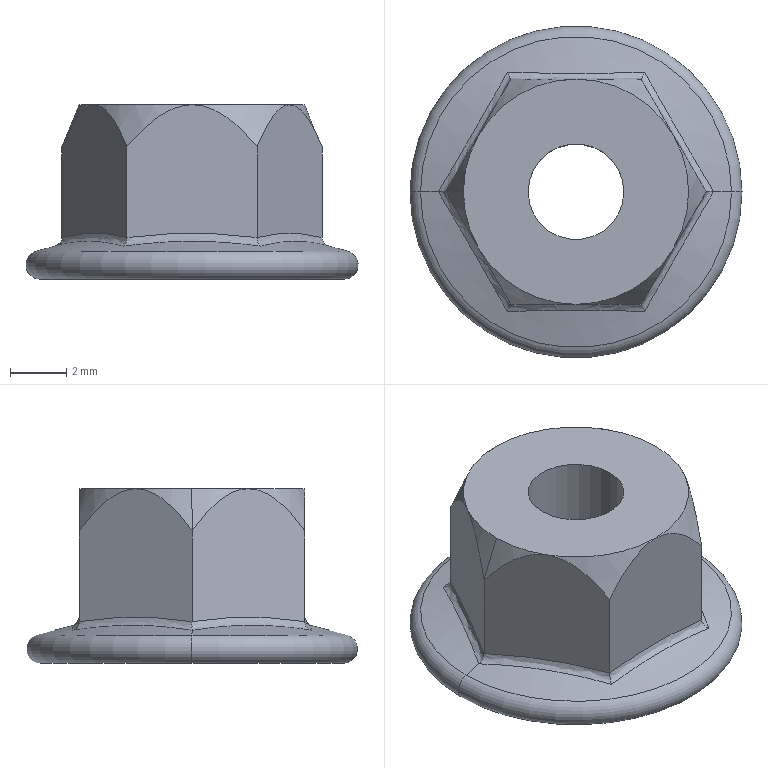Part | SolidWorks | features BaseBody 1 | 1 solid | 29 faces | box 11.8 x 11.8 x 6.2 mm | volume 341.044 mm3 | cone 11 | plane 8 | spline 6 | torus 2 | cylinder 2 | commonest cylinder face diameters 3.4 x2
STEP:
#1=CARTESIAN_POINT('',(2.444,4.233,-5.03));
#2=VERTEX_POINT('',#1);
#3=CARTESIAN_POINT('',(4.888,0.,-5.03));
#4=VERTEX_POINT('',#3);
#5=CARTESIAN_POINT('',(2.444,4.233,-5.03));
#6=CARTESIAN_POINT('',(2.548,4.05,-5.001));
#7=CARTESIAN_POINT('',(2.649,3.872,-4.976));
#8=CARTESIAN_POINT('',(2.799,3.608,-4.943));
#9=CARTESIAN_POINT('',(2.849,3.521,-4.933));
#10=CARTESIAN_POINT('',(2.923,3.39,-4.92));
#11=CARTESIAN_POINT('',(2.96,3.325,-4.913));
#12=CARTESIAN_POINT('',(2.997,3.261,-4.907));
#13=CARTESIAN_POINT('',(3.022,3.217,-4.903));
#14=CARTESIAN_POINT('',(3.034,3.197,-4.901));
#15=CARTESIAN_POINT('',(3.254,2.812,-4.867));
#16=CARTESIAN_POINT('',(3.451,2.468,-4.852));
#17=CARTESIAN_POINT('',(3.758,1.935,-4.851));
#18=CARTESIAN_POINT('',(3.859,1.76,-4.855));
#19=CARTESIAN_POINT('',(4.012,1.497,-4.867));
#20=CARTESIAN_POINT('',(4.063,1.409,-4.872));
#21=CARTESIAN_POINT('',(4.141,1.276,-4.881));
#22=CARTESIAN_POINT('',(4.18,1.21,-4.886));
#23=CARTESIAN_POINT('',(4.219,1.143,-4.891));
#24=CARTESIAN_POINT('',(4.245,1.098,-4.895));
#25=CARTESIAN_POINT('',(4.259,1.074,-4.897));
#26=CARTESIAN_POINT('',(4.472,0.709,-4.929));
#27=CARTESIAN_POINT('',(4.675,0.3632,-4.973));
#28=CARTESIAN_POINT('',(4.888,0.,-5.03));
#29=B_SPLINE_CURVE_WITH_KNOTS('',3,(#5,#6,#7,#8,#9,#10,#11,#12,#13,#14,#15,#16,#17,#18,#19,#20,#21,#22,#23,#24,#25,#26,#27,#28),.UNSPECIFIED.,.F.,.F.,(4,2,2,1,2,2,2,2,2,1,2,2,4),(0.,0.125,0.1875,0.2187,0.2344,0.25,0.5,0.625,0.6875,0.7187,0.7344,0.75,1.),.UNSPECIFIED.);
#30=EDGE_CURVE('',#2,#4,#29,.T.);
#31=ORIENTED_EDGE('',*,*,#30,.T.);
#32=CARTESIAN_POINT('',(5.523,0.,-5.2));
#33=VERTEX_POINT('',#32);
#34=CARTESIAN_POINT('',(4.619,0.,-4.958));
#35=DIRECTION('',(0.9659,0.,-0.2588));
#36=VECTOR('',#35,1000.);
#37=LINE('',#34,#36);
#38=EDGE_CURVE('',#4,#33,#37,.T.);
#39=ORIENTED_EDGE('',*,*,#38,.T.);
#40=CARTESIAN_POINT('',(-5.523,0.,-5.2));
#41=VERTEX_POINT('',#40);
#42=CARTESIAN_POINT('',(0.,0.,-5.2));
#43=DIRECTION('',(0.,0.,-1.));
#44=DIRECTION('',(-1.,0.,0.));
#45=AXIS2_PLACEMENT_3D('',#42,#43,#44);
#46=CIRCLE('',#45,5.523);
#47=EDGE_CURVE('',#41,#33,#46,.T.);
#48=ORIENTED_EDGE('',*,*,#47,.F.);
#49=CARTESIAN_POINT('',(-4.888,0.,-5.03));
#50=VERTEX_POINT('',#49);
#51=CARTESIAN_POINT('',(-4.619,0.,-4.958));
#52=DIRECTION('',(-0.9659,0.,-0.2588));
#53=VECTOR('',#52,1000.);
#54=LINE('',#51,#53);
#55=EDGE_CURVE('',#50,#41,#54,.T.);
#56=ORIENTED_EDGE('',*,*,#55,.F.);
#57=CARTESIAN_POINT('',(-2.444,4.233,-5.03));
#58=VERTEX_POINT('',#57);
#59=CARTESIAN_POINT('',(-4.888,0.,-5.03));
#60=CARTESIAN_POINT('',(-4.781,0.1813,-5.001));
#61=CARTESIAN_POINT('',(-4.677,0.3583,-4.976));
#62=CARTESIAN_POINT('',(-4.524,0.6202,-4.943));
#63=CARTESIAN_POINT('',(-4.473,0.7069,-4.933));
#64=CARTESIAN_POINT('',(-4.398,0.8363,-4.92));
#65=CARTESIAN_POINT('',(-4.36,0.9009,-4.913));
#66=CARTESIAN_POINT('',(-4.322,0.9654,-4.907));
#67=CARTESIAN_POINT('',(-4.297,1.008,-4.903));
#68=CARTESIAN_POINT('',(-4.285,1.029,-4.901));
#69=CARTESIAN_POINT('',(-4.062,1.412,-4.867));
#70=CARTESIAN_POINT('',(-3.862,1.755,-4.852));
#71=CARTESIAN_POINT('',(-3.555,2.287,-4.851));
#72=CARTESIAN_POINT('',(-3.454,2.462,-4.855));
#73=CARTESIAN_POINT('',(-3.303,2.726,-4.867));
#74=CARTESIAN_POINT('',(-3.252,2.814,-4.872));
#75=CARTESIAN_POINT('',(-3.176,2.948,-4.881));
#76=CARTESIAN_POINT('',(-3.138,3.015,-4.886));
#77=CARTESIAN_POINT('',(-3.099,3.082,-4.891));
#78=CARTESIAN_POINT('',(-3.073,3.127,-4.895));
#79=CARTESIAN_POINT('',(-3.06,3.151,-4.897));
#80=CARTESIAN_POINT('',(-2.85,3.518,-4.929));
#81=CARTESIAN_POINT('',(-2.652,3.867,-4.973));
#82=CARTESIAN_POINT('',(-2.444,4.233,-5.03));
#83=B_SPLINE_CURVE_WITH_KNOTS('',3,(#59,#60,#61,#62,#63,#64,#65,#66,#67,#68,#69,#70,#71,#72,#73,#74,#75,#76,#77,#78,#79,#80,#81,#82),.UNSPECIFIED.,.F.,.F.,(4,2,2,1,2,2,2,2,2,1,2,2,4),(0.,0.125,0.1875,0.2187,0.2344,0.25,0.5,0.625,0.6875,0.7187,0.7344,0.75,1.),.UNSPECIFIED.);
#84=EDGE_CURVE('',#50,#58,#83,.T.);
#85=ORIENTED_EDGE('',*,*,#84,.T.);
#86=CARTESIAN_POINT('',(-2.444,4.233,-5.03));
#87=CARTESIAN_POINT('',(-2.234,4.231,-5.001));
#88=CARTESIAN_POINT('',(-2.028,4.23,-4.976));
#89=CARTESIAN_POINT('',(-1.725,4.228,-4.943));
#90=CARTESIAN_POINT('',(-1.625,4.228,-4.933));
#91=CARTESIAN_POINT('',(-1.475,4.227,-4.92));
#92=CARTESIAN_POINT('',(-1.4,4.226,-4.913));
#93=CARTESIAN_POINT('',(-1.325,4.226,-4.907));
#94=CARTESIAN_POINT('',(-1.275,4.226,-4.903));
#95=CARTESIAN_POINT('',(-1.252,4.226,-4.901));
#96=CARTESIAN_POINT('',(-0.8085,4.224,-4.867));
#97=CARTESIAN_POINT('',(-0.4116,4.222,-4.852));
#98=CARTESIAN_POINT('',(0.2033,4.222,-4.851));
#99=CARTESIAN_POINT('',(0.4052,4.222,-4.855));
#100=CARTESIAN_POINT('',(0.7095,4.223,-4.867));
#101=CARTESIAN_POINT('',(0.8112,4.224,-4.872));
#102=CARTESIAN_POINT('',(0.965,4.224,-4.881));
#103=CARTESIAN_POINT('',(1.042,4.225,-4.886));
#104=CARTESIAN_POINT('',(1.12,4.225,-4.891));
#105=CARTESIAN_POINT('',(1.172,4.225,-4.895));
#106=CARTESIAN_POINT('',(1.199,4.225,-4.897));
#107=CARTESIAN_POINT('',(1.622,4.227,-4.929));
#108=CARTESIAN_POINT('',(2.023,4.23,-4.973));
#109=CARTESIAN_POINT('',(2.444,4.233,-5.03));
#110=B_SPLINE_CURVE_WITH_KNOTS('',3,(#86,#87,#88,#89,#90,#91,#92,#93,#94,#95,#96,#97,#98,#99,#100,#101,#102,#103,#104,#105,#106,#107,#108,#109),.UNSPECIFIED.,.F.,.F.,(4,2,2,1,2,2,2,2,2,1,2,2,4),(0.,0.125,0.1875,0.2188,0.2344,0.25,0.5,0.625,0.6875,0.7188,0.7344,0.75,1.),.UNSPECIFIED.);
#111=EDGE_CURVE('',#58,#2,#110,.T.);
#112=ORIENTED_EDGE('',*,*,#111,.T.);
#113=EDGE_LOOP('',(#31,#39,#48,#56,#85,#112));
#114=FACE_OUTER_BOUND('',#113,.T.);
#115=CARTESIAN_POINT('',(0.,0.,-4.958));
#116=DIRECTION('',(0.,0.,-1.));
#117=DIRECTION('',(-1.,0.,0.));
#118=AXIS2_PLACEMENT_3D('',#115,#116,#117);
#119=CONICAL_SURFACE('',#118,4.619,1.309);
#120=ADVANCED_FACE('',(#114),#119,.T.);
#121=ORIENTED_EDGE('',*,*,#47,.T.);
#122=CARTESIAN_POINT('',(5.391,0.,-6.2));
#123=VERTEX_POINT('',#122);
#124=CARTESIAN_POINT('',(5.391,0.,-5.691));
#125=DIRECTION('',(0.,1.,0.));
#126=DIRECTION('',(-1.,0.,0.));
#127=AXIS2_PLACEMENT_3D('',#124,#125,#126);
#128=CIRCLE('',#127,0.5087);
#129=EDGE_CURVE('',#33,#123,#128,.T.);
#130=ORIENTED_EDGE('',*,*,#129,.T.);
#131=CARTESIAN_POINT('',(-5.391,0.,-6.2));
#132=VERTEX_POINT('',#131);
#133=CARTESIAN_POINT('',(0.,0.,-6.2));
#134=DIRECTION('',(0.,0.,-1.));
#135=DIRECTION('',(-1.,0.,0.));
#136=AXIS2_PLACEMENT_3D('',#133,#134,#135);
#137=CIRCLE('',#136,5.391);
#138=EDGE_CURVE('',#132,#123,#137,.T.);
#139=ORIENTED_EDGE('',*,*,#138,.F.);
#140=CARTESIAN_POINT('',(-5.391,0.,-5.691));
#141=DIRECTION('',(0.,-1.,0.));
#142=DIRECTION('',(0.,0.,-1.));
#143=AXIS2_PLACEMENT_3D('',#140,#141,#142);
#144=CIRCLE('',#143,0.5087);
#145=EDGE_CURVE('',#41,#132,#144,.T.);
#146=ORIENTED_EDGE('',*,*,#145,.F.);
#147=EDGE_LOOP('',(#121,#130,#139,#146));
#148=FACE_OUTER_BOUND('',#147,.T.);
#149=CARTESIAN_POINT('',(0.,0.,-5.691));
#150=DIRECTION('',(0.,0.,-1.));
#151=DIRECTION('',(-1.,0.,0.));
#152=AXIS2_PLACEMENT_3D('',#149,#150,#151);
#153=TOROIDAL_SURFACE('',#152,5.391,0.5087);
#154=ADVANCED_FACE('',(#148),#153,.T.);
#155=CARTESIAN_POINT('',(1.7,0.,-5.714));
#156=VERTEX_POINT('',#155);
#157=CARTESIAN_POINT('',(-1.7,0.,-5.714));
#158=VERTEX_POINT('',#157);
#159=CARTESIAN_POINT('',(0.,0.,-5.714));
#160=DIRECTION('',(0.,0.,-1.));
#161=DIRECTION('',(1.,0.,0.));
#162=AXIS2_PLACEMENT_3D('',#159,#160,#161);
#163=CIRCLE('',#162,1.7);
#164=EDGE_CURVE('',#156,#158,#163,.T.);
#165=ORIENTED_EDGE('',*,*,#164,.F.);
#166=CARTESIAN_POINT('',(2.186,0.,-6.2));
#167=VERTEX_POINT('',#166);
#168=CARTESIAN_POINT('',(2.186,0.,-6.2));
#169=DIRECTION('',(0.7071,0.,-0.7071));
#170=VECTOR('',#169,1000.);
#171=LINE('',#168,#170);
#172=EDGE_CURVE('',#156,#167,#171,.T.);
#173=ORIENTED_EDGE('',*,*,#172,.T.);
#174=CARTESIAN_POINT('',(-2.186,0.,-6.2));
#175=VERTEX_POINT('',#174);
#176=CARTESIAN_POINT('',(0.,0.,-6.2));
#177=DIRECTION('',(0.,0.,1.));
#178=DIRECTION('',(1.,0.,0.));
#179=AXIS2_PLACEMENT_3D('',#176,#177,#178);
#180=CIRCLE('',#179,2.186);
#181=EDGE_CURVE('',#175,#167,#180,.T.);
#182=ORIENTED_EDGE('',*,*,#181,.F.);
#183=CARTESIAN_POINT('',(-2.186,0.,-6.2));
#184=DIRECTION('',(-0.7071,0.,-0.7071));
#185=VECTOR('',#184,1000.);
#186=LINE('',#183,#185);
#187=EDGE_CURVE('',#158,#175,#186,.T.);
#188=ORIENTED_EDGE('',*,*,#187,.F.);
#189=EDGE_LOOP('',(#165,#173,#182,#188));
#190=FACE_OUTER_BOUND('',#189,.T.);
#191=CARTESIAN_POINT('',(0.,0.,-6.2));
#192=DIRECTION('',(0.,0.,-1.));
#193=DIRECTION('',(-1.,0.,0.));
#194=AXIS2_PLACEMENT_3D('',#191,#192,#193);
#195=CONICAL_SURFACE('',#194,2.186,0.7854);
#196=ADVANCED_FACE('',(#190),#195,.F.);
#197=ORIENTED_EDGE('',*,*,#164,.T.);
#198=CARTESIAN_POINT('',(-1.7,0.,0.));
#199=VERTEX_POINT('',#198);
#200=CARTESIAN_POINT('',(-1.7,0.,-6.2));
#201=DIRECTION('',(0.,0.,1.));
#202=VECTOR('',#201,1000.);
#203=LINE('',#200,#202);
#204=EDGE_CURVE('',#158,#199,#203,.T.);
#205=ORIENTED_EDGE('',*,*,#204,.T.);
#206=CARTESIAN_POINT('',(1.7,0.,0.));
#207=VERTEX_POINT('',#206);
#208=CARTESIAN_POINT('',(0.,0.,0.));
#209=DIRECTION('',(0.,0.,1.));
#210=DIRECTION('',(1.,0.,0.));
#211=AXIS2_PLACEMENT_3D('',#208,#209,#210);
#212=CIRCLE('',#211,1.7);
#213=EDGE_CURVE('',#199,#207,#212,.T.);
#214=ORIENTED_EDGE('',*,*,#213,.T.);
#215=CARTESIAN_POINT('',(1.7,0.,-6.2));
#216=DIRECTION('',(0.,0.,1.));
#217=VECTOR('',#216,1000.);
#218=LINE('',#215,#217);
#219=EDGE_CURVE('',#156,#207,#218,.T.);
#220=ORIENTED_EDGE('',*,*,#219,.F.);
#221=EDGE_LOOP('',(#197,#205,#214,#220));
#222=FACE_OUTER_BOUND('',#221,.T.);
#223=CARTESIAN_POINT('',(0.,0.,-6.2));
#224=DIRECTION('',(0.,0.,1.));
#225=DIRECTION('',(1.,0.,0.));
#226=AXIS2_PLACEMENT_3D('',#223,#224,#225);
#227=CYLINDRICAL_SURFACE('',#226,1.7);
#228=ADVANCED_FACE('',(#222),#227,.F.);
#229=CARTESIAN_POINT('',(-3.464,-2.,0.));
#230=VERTEX_POINT('',#229);
#231=CARTESIAN_POINT('',(-4.,0.,0.));
#232=VERTEX_POINT('',#231);
#233=CARTESIAN_POINT('',(0.,0.,0.));
#234=DIRECTION('',(0.,0.,-1.));
#235=DIRECTION('',(1.,0.,0.));
#236=AXIS2_PLACEMENT_3D('',#233,#234,#235);
#237=CIRCLE('',#236,4.);
#238=EDGE_CURVE('',#230,#232,#237,.T.);
#239=ORIENTED_EDGE('',*,*,#238,.T.);
#240=CARTESIAN_POINT('',(-4.619,0.,-1.5));
#241=VERTEX_POINT('',#240);
#242=CARTESIAN_POINT('',(-4.,0.,0.));
#243=DIRECTION('',(-0.3814,0.,-0.9244));
#244=VECTOR('',#243,1000.);
#245=LINE('',#242,#244);
#246=EDGE_CURVE('',#232,#241,#245,.T.);
#247=ORIENTED_EDGE('',*,*,#246,.T.);
#248=CARTESIAN_POINT('',(-4.619,0.,-1.5));
#249=CARTESIAN_POINT('',(-4.543,-0.1306,-1.317));
#250=CARTESIAN_POINT('',(-4.465,-0.2661,-1.141));
#251=CARTESIAN_POINT('',(-4.3,-0.5524,-0.8063));
#252=CARTESIAN_POINT('',(-4.213,-0.703,-0.6482));
#253=CARTESIAN_POINT('',(-4.024,-1.03,-0.3637));
#254=CARTESIAN_POINT('',(-3.922,-1.208,-0.2367));
#255=CARTESIAN_POINT('',(-3.703,-1.587,-0.05468));
#256=CARTESIAN_POINT('',(-3.584,-1.792,0.));
#257=CARTESIAN_POINT('',(-3.464,-2.,0.));
#258=B_SPLINE_CURVE_WITH_KNOTS('',3,(#248,#249,#250,#251,#252,#253,#254,#255,#256,#257),.UNSPECIFIED.,.F.,.F.,(4,2,2,2,4),(0.,0.0007048,0.00141,0.002115,0.002819),.UNSPECIFIED.);
#259=EDGE_CURVE('',#241,#230,#258,.T.);
#260=ORIENTED_EDGE('',*,*,#259,.T.);
#261=EDGE_LOOP('',(#239,#247,#260));
#262=FACE_OUTER_BOUND('',#261,.T.);
#263=CARTESIAN_POINT('',(0.,0.,0.));
#264=DIRECTION('',(0.,0.,-1.));
#265=DIRECTION('',(-1.,0.,0.));
#266=AXIS2_PLACEMENT_3D('',#263,#264,#265);
#267=CONICAL_SURFACE('',#266,4.,0.3913);
#268=ADVANCED_FACE('',(#262),#267,.T.);
#269=CARTESIAN_POINT('',(-4.619,0.,-4.717));
#270=VERTEX_POINT('',#269);
#271=CARTESIAN_POINT('',(-4.888,0.,-5.03));
#272=CARTESIAN_POINT('',(-4.853,0.,-5.021));
#273=CARTESIAN_POINT('',(-4.818,-0.000409,-5.006));
#274=CARTESIAN_POINT('',(-4.77,0.0002124,-4.977));
#275=CARTESIAN_POINT('',(-4.755,0.000207,-4.967));
#276=CARTESIAN_POINT('',(-4.733,0.0001255,-4.949));
#277=CARTESIAN_POINT('',(-4.726,0.00008611,-4.943));
#278=CARTESIAN_POINT('',(-4.713,0.00002162,-4.931));
#279=CARTESIAN_POINT('',(-4.707,-0.000003411,-4.925));
#280=CARTESIAN_POINT('',(-4.644,-0.000002588,-4.855));
#281=CARTESIAN_POINT('',(-4.619,0.000006557,-4.78));
#282=CARTESIAN_POINT('',(-4.619,0.,-4.717));
#283=B_SPLINE_CURVE_WITH_KNOTS('',3,(#271,#272,#273,#274,#275,#276,#277,#278,#279,#280,#281,#282),.UNSPECIFIED.,.F.,.F.,(4,2,2,2,2,4),(0.,0.25,0.375,0.4375,0.5,1.),.UNSPECIFIED.);
#284=EDGE_CURVE('',#50,#270,#283,.T.);
#285=ORIENTED_EDGE('',*,*,#284,.T.);
#286=CARTESIAN_POINT('',(-2.309,4.,-4.717));
#287=VERTEX_POINT('',#286);
#288=CARTESIAN_POINT('',(-2.309,4.,-4.717));
#289=CARTESIAN_POINT('',(-2.693,3.336,-4.62));
#290=CARTESIAN_POINT('',(-3.077,2.67,-4.562));
#291=CARTESIAN_POINT('',(-3.851,1.33,-4.562));
#292=CARTESIAN_POINT('',(-4.235,0.664,-4.62));
#293=CARTESIAN_POINT('',(-4.619,0.,-4.717));
#294=B_SPLINE_CURVE_WITH_KNOTS('',3,(#288,#289,#290,#291,#292,#293),.UNSPECIFIED.,.F.,.F.,(4,2,4),(0.,0.002315,0.004629),.UNSPECIFIED.);
#295=EDGE_CURVE('',#287,#270,#294,.T.);
#296=ORIENTED_EDGE('',*,*,#295,.F.);
#297=CARTESIAN_POINT('',(-2.309,4.,-4.717));
#298=CARTESIAN_POINT('',(-2.309,4.,-4.749));
#299=CARTESIAN_POINT('',(-2.312,4.005,-4.783));
#300=CARTESIAN_POINT('',(-2.322,4.023,-4.835));
#301=CARTESIAN_POINT('',(-2.326,4.03,-4.852));
#302=CARTESIAN_POINT('',(-2.334,4.043,-4.877));
#303=CARTESIAN_POINT('',(-2.339,4.051,-4.89));
#304=CARTESIAN_POINT('',(-2.344,4.06,-4.904));
#305=CARTESIAN_POINT('',(-2.347,4.065,-4.91));
#306=CARTESIAN_POINT('',(-2.348,4.068,-4.914));
#307=CARTESIAN_POINT('',(-2.35,4.07,-4.917));
#308=CARTESIAN_POINT('',(-2.355,4.079,-4.929));
#309=CARTESIAN_POINT('',(-2.364,4.096,-4.948));
#310=CARTESIAN_POINT('',(-2.395,4.148,-4.991));
#311=CARTESIAN_POINT('',(-2.417,4.185,-5.015));
#312=CARTESIAN_POINT('',(-2.444,4.233,-5.03));
#313=B_SPLINE_CURVE_WITH_KNOTS('',3,(#297,#298,#299,#300,#301,#302,#303,#304,#305,#306,#307,#308,#309,#310,#311,#312),.UNSPECIFIED.,.F.,.F.,(4,2,2,1,1,2,2,2,4),(0.,0.25,0.375,0.4375,0.4688,0.4844,0.5,0.75,1.),.UNSPECIFIED.);
#314=EDGE_CURVE('',#287,#58,#313,.T.);
#315=ORIENTED_EDGE('',*,*,#314,.T.);
#316=ORIENTED_EDGE('',*,*,#84,.F.);
#317=EDGE_LOOP('',(#285,#296,#315,#316));
#318=FACE_OUTER_BOUND('',#317,.T.);
#319=CARTESIAN_POINT('',(-2.208,4.175,-4.744));
#320=CARTESIAN_POINT('',(-2.224,4.148,-4.981));
#321=CARTESIAN_POINT('',(-2.429,4.258,-5.034));
#322=CARTESIAN_POINT('',(-2.62,3.463,-4.633));
#323=CARTESIAN_POINT('',(-2.628,3.447,-4.867));
#324=CARTESIAN_POINT('',(-2.831,3.551,-4.922));
#325=CARTESIAN_POINT('',(-3.036,2.742,-4.562));
#326=CARTESIAN_POINT('',(-3.042,2.732,-4.792));
#327=CARTESIAN_POINT('',(-3.236,2.84,-4.852));
#328=CARTESIAN_POINT('',(-3.883,1.275,-4.561));
#329=CARTESIAN_POINT('',(-3.877,1.285,-4.791));
#330=CARTESIAN_POINT('',(-4.068,1.399,-4.851));
#331=CARTESIAN_POINT('',(-4.303,0.5472,-4.631));
#332=CARTESIAN_POINT('',(-4.294,0.5622,-4.865));
#333=CARTESIAN_POINT('',(-4.485,0.6866,-4.921));
#334=CARTESIAN_POINT('',(-4.72,-0.1757,-4.744));
#335=CARTESIAN_POINT('',(-4.704,-0.148,-4.981));
#336=CARTESIAN_POINT('',(-4.902,-0.02532,-5.034));
#337=(BOUNDED_SURFACE()B_SPLINE_SURFACE(3,2,((#319,#320,#321),(#322,#323,#324),(#325,#326,#327),(#328,#329,#330),(#331,#332,#333),(#334,#335,#336)),.UNSPECIFIED.,.F.,.F.,.T.)B_SPLINE_SURFACE_WITH_KNOTS((4,2,4),(3,3),(0.0205,0.02298,0.02547),(0.,1.),.UNSPECIFIED.)GEOMETRIC_REPRESENTATION_ITEM()RATIONAL_B_SPLINE_SURFACE(((1.,0.7821,1.),(1.,0.7882,1.),(1.,0.7933,1.),(1.,0.7934,1.),(1.,0.7883,1.),(1.,0.7821,1.)))REPRESENTATION_ITEM('')SURFACE());
#338=ADVANCED_FACE('',(#318),#337,.F.);
#339=CARTESIAN_POINT('',(2.309,4.,-4.717));
#340=VERTEX_POINT('',#339);
#341=CARTESIAN_POINT('',(2.309,4.,-4.717));
#342=CARTESIAN_POINT('',(2.309,4.,-4.749));
#343=CARTESIAN_POINT('',(2.313,4.005,-4.783));
#344=CARTESIAN_POINT('',(2.323,4.022,-4.835));
#345=CARTESIAN_POINT('',(2.327,4.03,-4.852));
#346=CARTESIAN_POINT('',(2.335,4.043,-4.877));
#347=CARTESIAN_POINT('',(2.339,4.051,-4.89));
#348=CARTESIAN_POINT('',(2.344,4.06,-4.904));
#349=CARTESIAN_POINT('',(2.347,4.065,-4.91));
#350=CARTESIAN_POINT('',(2.348,4.068,-4.914));
#351=CARTESIAN_POINT('',(2.35,4.07,-4.917));
#352=CARTESIAN_POINT('',(2.355,4.079,-4.929));
#353=CARTESIAN_POINT('',(2.365,4.095,-4.948));
#354=CARTESIAN_POINT('',(2.395,4.148,-4.991));
#355=CARTESIAN_POINT('',(2.416,4.186,-5.015));
#356=CARTESIAN_POINT('',(2.444,4.233,-5.03));
#357=B_SPLINE_CURVE_WITH_KNOTS('',3,(#341,#342,#343,#344,#345,#346,#347,#348,#349,#350,#351,#352,#353,#354,#355,#356),.UNSPECIFIED.,.F.,.F.,(4,2,2,1,1,2,2,2,4),(0.,0.25,0.375,0.4375,0.4687,0.4844,0.5,0.75,1.),.UNSPECIFIED.);
#358=EDGE_CURVE('',#340,#2,#357,.T.);
#359=ORIENTED_EDGE('',*,*,#358,.T.);
#360=ORIENTED_EDGE('',*,*,#111,.F.);
#361=ORIENTED_EDGE('',*,*,#314,.F.);
#362=CARTESIAN_POINT('',(2.309,4.,-4.717));
#363=CARTESIAN_POINT('',(1.543,4.,-4.62));
#364=CARTESIAN_POINT('',(0.7733,4.,-4.562));
#365=CARTESIAN_POINT('',(-0.7733,4.,-4.562));
#366=CARTESIAN_POINT('',(-1.543,4.,-4.62));
#367=CARTESIAN_POINT('',(-2.309,4.,-4.717));
#368=B_SPLINE_CURVE_WITH_KNOTS('',3,(#362,#363,#364,#365,#366,#367),.UNSPECIFIED.,.F.,.F.,(4,2,4),(0.,0.002315,0.004629),.UNSPECIFIED.);
#369=EDGE_CURVE('',#340,#287,#368,.T.);
#370=ORIENTED_EDGE('',*,*,#369,.F.);
#371=EDGE_LOOP('',(#359,#360,#361,#370));
#372=FACE_OUTER_BOUND('',#371,.T.);
#373=CARTESIAN_POINT('',(2.512,4.,-4.744));
#374=CARTESIAN_POINT('',(2.48,4.,-4.981));
#375=CARTESIAN_POINT('',(2.473,4.233,-5.034));
#376=CARTESIAN_POINT('',(1.689,4.,-4.633));
#377=CARTESIAN_POINT('',(1.671,4.,-4.867));
#378=CARTESIAN_POINT('',(1.659,4.227,-4.922));
#379=CARTESIAN_POINT('',(0.8571,4.,-4.562));
#380=CARTESIAN_POINT('',(0.8448,4.,-4.792));
#381=CARTESIAN_POINT('',(0.8416,4.222,-4.852));
#382=CARTESIAN_POINT('',(-0.8378,4.,-4.561));
#383=CARTESIAN_POINT('',(-0.8257,4.,-4.791));
#384=CARTESIAN_POINT('',(-0.8227,4.222,-4.851));
#385=CARTESIAN_POINT('',(-1.678,4.,-4.631));
#386=CARTESIAN_POINT('',(-1.66,4.,-4.865));
#387=CARTESIAN_POINT('',(-1.648,4.227,-4.921));
#388=CARTESIAN_POINT('',(-2.512,4.,-4.744));
#389=CARTESIAN_POINT('',(-2.48,4.,-4.981));
#390=CARTESIAN_POINT('',(-2.473,4.233,-5.034));
#391=(BOUNDED_SURFACE()B_SPLINE_SURFACE(3,2,((#373,#374,#375),(#376,#377,#378),(#379,#380,#381),(#382,#383,#384),(#385,#386,#387),(#388,#389,#390)),.UNSPECIFIED.,.F.,.F.,.T.)B_SPLINE_SURFACE_WITH_KNOTS((4,2,4),(3,3),(0.02046,0.02295,0.02543),(0.,1.),.UNSPECIFIED.)GEOMETRIC_REPRESENTATION_ITEM()RATIONAL_B_SPLINE_SURFACE(((1.,0.7821,1.),(1.,0.7882,1.),(1.,0.7933,1.),(1.,0.7934,1.),(1.,0.7883,1.),(1.,0.7821,1.)))REPRESENTATION_ITEM('')SURFACE());
#392=ADVANCED_FACE('',(#372),#391,.F.);
#393=CARTESIAN_POINT('',(-2.444,-4.233,-5.03));
#394=VERTEX_POINT('',#393);
#395=CARTESIAN_POINT('',(-2.309,-4.,-4.717));
#396=VERTEX_POINT('',#395);
#397=CARTESIAN_POINT('',(-2.444,-4.233,-5.03));
#398=CARTESIAN_POINT('',(-2.427,-4.203,-5.021));
#399=CARTESIAN_POINT('',(-2.408,-4.172,-5.006));
#400=CARTESIAN_POINT('',(-2.385,-4.131,-4.977));
#401=CARTESIAN_POINT('',(-2.377,-4.117,-4.967));
#402=CARTESIAN_POINT('',(-2.367,-4.099,-4.949));
#403=CARTESIAN_POINT('',(-2.363,-4.093,-4.943));
#404=CARTESIAN_POINT('',(-2.356,-4.081,-4.931));
#405=CARTESIAN_POINT('',(-2.354,-4.077,-4.925));
#406=CARTESIAN_POINT('',(-2.322,-4.022,-4.855));
#407=CARTESIAN_POINT('',(-2.309,-4.,-4.78));
#408=CARTESIAN_POINT('',(-2.309,-4.,-4.717));
#409=B_SPLINE_CURVE_WITH_KNOTS('',3,(#397,#398,#399,#400,#401,#402,#403,#404,#405,#406,#407,#408),.UNSPECIFIED.,.F.,.F.,(4,2,2,2,2,4),(0.,0.25,0.375,0.4375,0.5,1.),.UNSPECIFIED.);
#410=EDGE_CURVE('',#394,#396,#409,.T.);
#411=ORIENTED_EDGE('',*,*,#410,.T.);
#412=CARTESIAN_POINT('',(-4.619,0.,-4.717));
#413=CARTESIAN_POINT('',(-4.235,-0.664,-4.62));
#414=CARTESIAN_POINT('',(-3.851,-1.33,-4.562));
#415=CARTESIAN_POINT('',(-3.077,-2.67,-4.562));
#416=CARTESIAN_POINT('',(-2.693,-3.336,-4.62));
#417=CARTESIAN_POINT('',(-2.309,-4.,-4.717));
#418=B_SPLINE_CURVE_WITH_KNOTS('',3,(#412,#413,#414,#415,#416,#417),.UNSPECIFIED.,.F.,.F.,(4,2,4),(0.,0.002315,0.004629),.UNSPECIFIED.);
#419=EDGE_CURVE('',#270,#396,#418,.T.);
#420=ORIENTED_EDGE('',*,*,#419,.F.);
#421=ORIENTED_EDGE('',*,*,#284,.F.);
#422=CARTESIAN_POINT('',(-2.444,-4.233,-5.03));
#423=CARTESIAN_POINT('',(-2.548,-4.05,-5.001));
#424=CARTESIAN_POINT('',(-2.649,-3.872,-4.976));
#425=CARTESIAN_POINT('',(-2.799,-3.608,-4.943));
#426=CARTESIAN_POINT('',(-2.849,-3.521,-4.933));
#427=CARTESIAN_POINT('',(-2.923,-3.39,-4.92));
#428=CARTESIAN_POINT('',(-2.96,-3.325,-4.913));
#429=CARTESIAN_POINT('',(-2.997,-3.261,-4.907));
#430=CARTESIAN_POINT('',(-3.022,-3.217,-4.903));
#431=CARTESIAN_POINT('',(-3.034,-3.197,-4.901));
#432=CARTESIAN_POINT('',(-3.254,-2.812,-4.867));
#433=CARTESIAN_POINT('',(-3.451,-2.468,-4.852));
#434=CARTESIAN_POINT('',(-3.758,-1.935,-4.851));
#435=CARTESIAN_POINT('',(-3.859,-1.76,-4.855));
#436=CARTESIAN_POINT('',(-4.012,-1.497,-4.867));
#437=CARTESIAN_POINT('',(-4.063,-1.409,-4.872));
#438=CARTESIAN_POINT('',(-4.141,-1.276,-4.881));
#439=CARTESIAN_POINT('',(-4.18,-1.21,-4.886));
#440=CARTESIAN_POINT('',(-4.219,-1.143,-4.891));
#441=CARTESIAN_POINT('',(-4.245,-1.098,-4.895));
#442=CARTESIAN_POINT('',(-4.259,-1.074,-4.897));
#443=CARTESIAN_POINT('',(-4.472,-0.709,-4.929));
#444=CARTESIAN_POINT('',(-4.675,-0.3632,-4.973));
#445=CARTESIAN_POINT('',(-4.888,0.,-5.03));
#446=B_SPLINE_CURVE_WITH_KNOTS('',3,(#422,#423,#424,#425,#426,#427,#428,#429,#430,#431,#432,#433,#434,#435,#436,#437,#438,#439,#440,#441,#442,#443,#444,#445),.UNSPECIFIED.,.F.,.F.,(4,2,2,1,2,2,2,2,2,1,2,2,4),(0.,0.125,0.1875,0.2188,0.2344,0.25,0.5,0.625,0.6875,0.7188,0.7344,0.75,1.),.UNSPECIFIED.);
#447=EDGE_CURVE('',#394,#50,#446,.T.);
#448=ORIENTED_EDGE('',*,*,#447,.F.);
#449=EDGE_LOOP('',(#411,#420,#421,#448));
#450=FACE_OUTER_BOUND('',#449,.T.);
#451=CARTESIAN_POINT('',(-4.72,0.1754,-4.744));
#452=CARTESIAN_POINT('',(-4.704,0.1476,-4.981));
#453=CARTESIAN_POINT('',(-4.902,0.02496,-5.034));
#454=CARTESIAN_POINT('',(-4.309,-0.5372,-4.633));
#455=CARTESIAN_POINT('',(-4.3,-0.5525,-4.867));
#456=CARTESIAN_POINT('',(-4.491,-0.6768,-4.922));
#457=CARTESIAN_POINT('',(-3.893,-1.258,-4.562));
#458=CARTESIAN_POINT('',(-3.887,-1.268,-4.792));
#459=CARTESIAN_POINT('',(-4.078,-1.382,-4.852));
#460=CARTESIAN_POINT('',(-3.045,-2.725,-4.561));
#461=CARTESIAN_POINT('',(-3.051,-2.715,-4.791));
#462=CARTESIAN_POINT('',(-3.245,-2.823,-4.851));
#463=CARTESIAN_POINT('',(-2.625,-3.453,-4.631));
#464=CARTESIAN_POINT('',(-2.634,-3.438,-4.865));
#465=CARTESIAN_POINT('',(-2.837,-3.541,-4.921));
#466=CARTESIAN_POINT('',(-2.208,-4.176,-4.744));
#467=CARTESIAN_POINT('',(-2.224,-4.148,-4.981));
#468=CARTESIAN_POINT('',(-2.429,-4.258,-5.034));
#469=(BOUNDED_SURFACE()B_SPLINE_SURFACE(3,2,((#451,#452,#453),(#454,#455,#456),(#457,#458,#459),(#460,#461,#462),(#463,#464,#465),(#466,#467,#468)),.UNSPECIFIED.,.F.,.F.,.T.)B_SPLINE_SURFACE_WITH_KNOTS((4,2,4),(3,3),(0.0205,0.02298,0.02547),(0.,1.),.UNSPECIFIED.)GEOMETRIC_REPRESENTATION_ITEM()RATIONAL_B_SPLINE_SURFACE(((1.,0.7821,1.),(1.,0.7882,1.),(1.,0.7933,1.),(1.,0.7934,1.),(1.,0.7883,1.),(1.,0.7821,1.)))REPRESENTATION_ITEM('')SURFACE());
#470=ADVANCED_FACE('',(#450),#469,.F.);
#471=CARTESIAN_POINT('',(4.619,0.,-4.717));
#472=VERTEX_POINT('',#471);
#473=CARTESIAN_POINT('',(4.619,0.,-4.717));
#474=CARTESIAN_POINT('',(4.619,0.000005018,-4.749));
#475=CARTESIAN_POINT('',(4.625,-0.000302,-4.783));
#476=CARTESIAN_POINT('',(4.645,-0.0003222,-4.835));
#477=CARTESIAN_POINT('',(4.653,-0.0002683,-4.852));
#478=CARTESIAN_POINT('',(4.669,-0.0001491,-4.877));
#479=CARTESIAN_POINT('',(4.677,-0.00008204,-4.89));
#480=CARTESIAN_POINT('',(4.688,-0.00002565,-4.904));
#481=CARTESIAN_POINT('',(4.694,-0.0000114,-4.91));
#482=CARTESIAN_POINT('',(4.697,-0.00000472,-4.914));
#483=CARTESIAN_POINT('',(4.7,-0.000002661,-4.917));
#484=CARTESIAN_POINT('',(4.71,-0.000001503,-4.929));
#485=CARTESIAN_POINT('',(4.729,-0.0005767,-4.948));
#486=CARTESIAN_POINT('',(4.79,-0.0004463,-4.991));
#487=CARTESIAN_POINT('',(4.833,0.0006583,-5.015));
#488=CARTESIAN_POINT('',(4.888,0.,-5.03));
#489=B_SPLINE_CURVE_WITH_KNOTS('',3,(#473,#474,#475,#476,#477,#478,#479,#480,#481,#482,#483,#484,#485,#486,#487,#488),.UNSPECIFIED.,.F.,.F.,(4,2,2,1,1,2,2,2,4),(0.,0.25,0.375,0.4375,0.4688,0.4844,0.5,0.75,1.),.UNSPECIFIED.);
#490=EDGE_CURVE('',#472,#4,#489,.T.);
#491=ORIENTED_EDGE('',*,*,#490,.T.);
#492=ORIENTED_EDGE('',*,*,#30,.F.);
#493=ORIENTED_EDGE('',*,*,#358,.F.);
#494=CARTESIAN_POINT('',(4.619,0.,-4.717));
#495=CARTESIAN_POINT('',(4.235,0.664,-4.62));
#496=CARTESIAN_POINT('',(3.851,1.33,-4.562));
#497=CARTESIAN_POINT('',(3.077,2.67,-4.562));
#498=CARTESIAN_POINT('',(2.693,3.336,-4.62));
#499=CARTESIAN_POINT('',(2.309,4.,-4.717));
#500=B_SPLINE_CURVE_WITH_KNOTS('',3,(#494,#495,#496,#497,#498,#499),.UNSPECIFIED.,.F.,.F.,(4,2,4),(0.,0.002315,0.004629),.UNSPECIFIED.);
#501=EDGE_CURVE('',#472,#340,#500,.T.);
#502=ORIENTED_EDGE('',*,*,#501,.F.);
#503=EDGE_LOOP('',(#491,#492,#493,#502));
#504=FACE_OUTER_BOUND('',#503,.T.);
#505=CARTESIAN_POINT('',(4.72,-0.1754,-4.744));
#506=CARTESIAN_POINT('',(4.704,-0.1476,-4.981));
#507=CARTESIAN_POINT('',(4.902,-0.02496,-5.034));
#508=CARTESIAN_POINT('',(4.309,0.5372,-4.633));
#509=CARTESIAN_POINT('',(4.3,0.5525,-4.867));
#510=CARTESIAN_POINT('',(4.491,0.6768,-4.922));
#511=CARTESIAN_POINT('',(3.893,1.258,-4.562));
#512=CARTESIAN_POINT('',(3.887,1.268,-4.792));
#513=CARTESIAN_POINT('',(4.078,1.382,-4.852));
#514=CARTESIAN_POINT('',(3.045,2.725,-4.561));
#515=CARTESIAN_POINT('',(3.051,2.715,-4.791));
#516=CARTESIAN_POINT('',(3.245,2.823,-4.851));
#517=CARTESIAN_POINT('',(2.625,3.453,-4.631));
#518=CARTESIAN_POINT('',(2.634,3.438,-4.865));
#519=CARTESIAN_POINT('',(2.837,3.541,-4.921));
#520=CARTESIAN_POINT('',(2.208,4.176,-4.744));
#521=CARTESIAN_POINT('',(2.224,4.148,-4.981));
#522=CARTESIAN_POINT('',(2.429,4.258,-5.034));
#523=(BOUNDED_SURFACE()B_SPLINE_SURFACE(3,2,((#505,#506,#507),(#508,#509,#510),(#511,#512,#513),(#514,#515,#516),(#517,#518,#519),(#520,#521,#522)),.UNSPECIFIED.,.F.,.F.,.T.)B_SPLINE_SURFACE_WITH_KNOTS((4,2,4),(3,3),(0.0205,0.02298,0.02547),(0.,1.),.UNSPECIFIED.)GEOMETRIC_REPRESENTATION_ITEM()RATIONAL_B_SPLINE_SURFACE(((1.,0.7821,1.),(1.,0.7882,1.),(1.,0.7933,1.),(1.,0.7934,1.),(1.,0.7883,1.),(1.,0.7821,1.)))REPRESENTATION_ITEM('')SURFACE());
#524=ADVANCED_FACE('',(#504),#523,.F.);
#525=CARTESIAN_POINT('',(2.444,-4.233,-5.03));
#526=VERTEX_POINT('',#525);
#527=CARTESIAN_POINT('',(2.309,-4.,-4.717));
#528=VERTEX_POINT('',#527);
#529=CARTESIAN_POINT('',(2.444,-4.233,-5.03));
#530=CARTESIAN_POINT('',(2.427,-4.203,-5.021));
#531=CARTESIAN_POINT('',(2.409,-4.172,-5.006));
#532=CARTESIAN_POINT('',(2.385,-4.131,-4.977));
#533=CARTESIAN_POINT('',(2.377,-4.118,-4.967));
#534=CARTESIAN_POINT('',(2.366,-4.099,-4.949));
#535=CARTESIAN_POINT('',(2.363,-4.093,-4.943));
#536=CARTESIAN_POINT('',(2.356,-4.082,-4.931));
#537=CARTESIAN_POINT('',(2.354,-4.077,-4.925));
#538=CARTESIAN_POINT('',(2.322,-4.022,-4.855));
#539=CARTESIAN_POINT('',(2.309,-4.,-4.78));
#540=CARTESIAN_POINT('',(2.309,-4.,-4.717));
#541=B_SPLINE_CURVE_WITH_KNOTS('',3,(#529,#530,#531,#532,#533,#534,#535,#536,#537,#538,#539,#540),.UNSPECIFIED.,.F.,.F.,(4,2,2,2,2,4),(0.,0.25,0.375,0.4375,0.5,1.),.UNSPECIFIED.);
#542=EDGE_CURVE('',#526,#528,#541,.T.);
#543=ORIENTED_EDGE('',*,*,#542,.T.);
#544=CARTESIAN_POINT('',(-2.309,-4.,-4.717));
#545=CARTESIAN_POINT('',(-1.543,-4.,-4.62));
#546=CARTESIAN_POINT('',(-0.7733,-4.,-4.562));
#547=CARTESIAN_POINT('',(0.7733,-4.,-4.562));
#548=CARTESIAN_POINT('',(1.543,-4.,-4.62));
#549=CARTESIAN_POINT('',(2.309,-4.,-4.717));
#550=B_SPLINE_CURVE_WITH_KNOTS('',3,(#544,#545,#546,#547,#548,#549),.UNSPECIFIED.,.F.,.F.,(4,2,4),(0.,0.002315,0.004629),.UNSPECIFIED.);
#551=EDGE_CURVE('',#396,#528,#550,.T.);
#552=ORIENTED_EDGE('',*,*,#551,.F.);
#553=ORIENTED_EDGE('',*,*,#410,.F.);
#554=CARTESIAN_POINT('',(2.444,-4.233,-5.03));
#555=CARTESIAN_POINT('',(2.234,-4.231,-5.001));
#556=CARTESIAN_POINT('',(2.028,-4.23,-4.976));
#557=CARTESIAN_POINT('',(1.725,-4.228,-4.943));
#558=CARTESIAN_POINT('',(1.625,-4.228,-4.933));
#559=CARTESIAN_POINT('',(1.475,-4.227,-4.92));
#560=CARTESIAN_POINT('',(1.4,-4.226,-4.913));
#561=CARTESIAN_POINT('',(1.325,-4.226,-4.907));
#562=CARTESIAN_POINT('',(1.275,-4.226,-4.903));
#563=CARTESIAN_POINT('',(1.252,-4.226,-4.901));
#564=CARTESIAN_POINT('',(0.8085,-4.224,-4.867));
#565=CARTESIAN_POINT('',(0.4115,-4.222,-4.852));
#566=CARTESIAN_POINT('',(-0.2034,-4.222,-4.851));
#567=CARTESIAN_POINT('',(-0.4052,-4.222,-4.855));
#568=CARTESIAN_POINT('',(-0.7095,-4.223,-4.867));
#569=CARTESIAN_POINT('',(-0.8113,-4.224,-4.872));
#570=CARTESIAN_POINT('',(-0.965,-4.224,-4.881));
#571=CARTESIAN_POINT('',(-1.042,-4.225,-4.886));
#572=CARTESIAN_POINT('',(-1.12,-4.225,-4.891));
#573=CARTESIAN_POINT('',(-1.172,-4.225,-4.895));
#574=CARTESIAN_POINT('',(-1.199,-4.225,-4.897));
#575=CARTESIAN_POINT('',(-1.622,-4.227,-4.929));
#576=CARTESIAN_POINT('',(-2.023,-4.23,-4.973));
#577=CARTESIAN_POINT('',(-2.444,-4.233,-5.03));
#578=B_SPLINE_CURVE_WITH_KNOTS('',3,(#554,#555,#556,#557,#558,#559,#560,#561,#562,#563,#564,#565,#566,#567,#568,#569,#570,#571,#572,#573,#574,#575,#576,#577),.UNSPECIFIED.,.F.,.F.,(4,2,2,1,2,2,2,2,2,1,2,2,4),(0.,0.125,0.1875,0.2188,0.2344,0.25,0.5,0.625,0.6875,0.7188,0.7344,0.75,1.),.UNSPECIFIED.);
#579=EDGE_CURVE('',#526,#394,#578,.T.);
#580=ORIENTED_EDGE('',*,*,#579,.F.);
#581=EDGE_LOOP('',(#543,#552,#553,#580));
#582=FACE_OUTER_BOUND('',#581,.T.);
#583=CARTESIAN_POINT('',(-2.512,-4.,-4.744));
#584=CARTESIAN_POINT('',(-2.48,-4.,-4.981));
#585=CARTESIAN_POINT('',(-2.473,-4.233,-5.034));
#586=CARTESIAN_POINT('',(-1.689,-4.,-4.633));
#587=CARTESIAN_POINT('',(-1.671,-4.,-4.867));
#588=CARTESIAN_POINT('',(-1.659,-4.227,-4.922));
#589=CARTESIAN_POINT('',(-0.8572,-4.,-4.562));
#590=CARTESIAN_POINT('',(-0.8449,-4.,-4.792));
#591=CARTESIAN_POINT('',(-0.8417,-4.222,-4.852));
#592=CARTESIAN_POINT('',(0.8375,-4.,-4.561));
#593=CARTESIAN_POINT('',(0.8255,-4.,-4.791));
#594=CARTESIAN_POINT('',(0.8224,-4.222,-4.851));
#595=CARTESIAN_POINT('',(1.678,-4.,-4.631));
#596=CARTESIAN_POINT('',(1.66,-4.,-4.865));
#597=CARTESIAN_POINT('',(1.648,-4.227,-4.921));
#598=CARTESIAN_POINT('',(2.512,-4.,-4.744));
#599=CARTESIAN_POINT('',(2.48,-4.,-4.981));
#600=CARTESIAN_POINT('',(2.473,-4.233,-5.034));
#601=(BOUNDED_SURFACE()B_SPLINE_SURFACE(3,2,((#583,#584,#585),(#586,#587,#588),(#589,#590,#591),(#592,#593,#594),(#595,#596,#597),(#598,#599,#600)),.UNSPECIFIED.,.F.,.F.,.T.)B_SPLINE_SURFACE_WITH_KNOTS((4,2,4),(3,3),(0.02046,0.02294,0.02542),(0.,1.),.UNSPECIFIED.)GEOMETRIC_REPRESENTATION_ITEM()RATIONAL_B_SPLINE_SURFACE(((1.,0.7821,1.),(1.,0.7882,1.),(1.,0.7933,1.),(1.,0.7934,1.),(1.,0.7883,1.),(1.,0.7821,1.)))REPRESENTATION_ITEM('')SURFACE());
#602=ADVANCED_FACE('',(#582),#601,.F.);
#603=ORIENTED_EDGE('',*,*,#490,.F.);
#604=CARTESIAN_POINT('',(2.309,-4.,-4.717));
#605=CARTESIAN_POINT('',(2.693,-3.336,-4.62));
#606=CARTESIAN_POINT('',(3.077,-2.67,-4.562));
#607=CARTESIAN_POINT('',(3.851,-1.33,-4.562));
#608=CARTESIAN_POINT('',(4.235,-0.664,-4.62));
#609=CARTESIAN_POINT('',(4.619,0.,-4.717));
#610=B_SPLINE_CURVE_WITH_KNOTS('',3,(#604,#605,#606,#607,#608,#609),.UNSPECIFIED.,.F.,.F.,(4,2,4),(0.,0.002315,0.004629),.UNSPECIFIED.);
#611=EDGE_CURVE('',#528,#472,#610,.T.);
#612=ORIENTED_EDGE('',*,*,#611,.F.);
#613=ORIENTED_EDGE('',*,*,#542,.F.);
#614=CARTESIAN_POINT('',(4.888,0.,-5.03));
#615=CARTESIAN_POINT('',(4.781,-0.1813,-5.001));
#616=CARTESIAN_POINT('',(4.677,-0.3583,-4.976));
#617=CARTESIAN_POINT('',(4.524,-0.6202,-4.943));
#618=CARTESIAN_POINT('',(4.473,-0.7069,-4.933));
#619=CARTESIAN_POINT('',(4.398,-0.8363,-4.92));
#620=CARTESIAN_POINT('',(4.36,-0.9009,-4.913));
#621=CARTESIAN_POINT('',(4.322,-0.9654,-4.907));
#622=CARTESIAN_POINT('',(4.297,-1.008,-4.903));
#623=CARTESIAN_POINT('',(4.285,-1.029,-4.901));
#624=CARTESIAN_POINT('',(4.062,-1.412,-4.867));
#625=CARTESIAN_POINT('',(3.862,-1.755,-4.852));
#626=CARTESIAN_POINT('',(3.555,-2.287,-4.851));
#627=CARTESIAN_POINT('',(3.454,-2.462,-4.855));
#628=CARTESIAN_POINT('',(3.303,-2.726,-4.867));
#629=CARTESIAN_POINT('',(3.252,-2.814,-4.872));
#630=CARTESIAN_POINT('',(3.176,-2.948,-4.881));
#631=CARTESIAN_POINT('',(3.138,-3.015,-4.886));
#632=CARTESIAN_POINT('',(3.099,-3.082,-4.891));
#633=CARTESIAN_POINT('',(3.073,-3.127,-4.895));
#634=CARTESIAN_POINT('',(3.06,-3.151,-4.897));
#635=CARTESIAN_POINT('',(2.85,-3.518,-4.929));
#636=CARTESIAN_POINT('',(2.652,-3.867,-4.973));
#637=CARTESIAN_POINT('',(2.444,-4.233,-5.03));
#638=B_SPLINE_CURVE_WITH_KNOTS('',3,(#614,#615,#616,#617,#618,#619,#620,#621,#622,#623,#624,#625,#626,#627,#628,#629,#630,#631,#632,#633,#634,#635,#636,#637),.UNSPECIFIED.,.F.,.F.,(4,2,2,1,2,2,2,2,2,1,2,2,4),(0.,0.125,0.1875,0.2187,0.2344,0.25,0.5,0.625,0.6875,0.7188,0.7344,0.75,1.),.UNSPECIFIED.);
#639=EDGE_CURVE('',#4,#526,#638,.T.);
#640=ORIENTED_EDGE('',*,*,#639,.F.);
#641=EDGE_LOOP('',(#603,#612,#613,#640));
#642=FACE_OUTER_BOUND('',#641,.T.);
#643=CARTESIAN_POINT('',(2.208,-4.175,-4.744));
#644=CARTESIAN_POINT('',(2.224,-4.148,-4.981));
#645=CARTESIAN_POINT('',(2.429,-4.258,-5.034));
#646=CARTESIAN_POINT('',(2.62,-3.463,-4.633));
#647=CARTESIAN_POINT('',(2.628,-3.447,-4.867));
#648=CARTESIAN_POINT('',(2.831,-3.551,-4.922));
#649=CARTESIAN_POINT('',(3.036,-2.742,-4.562));
#650=CARTESIAN_POINT('',(3.042,-2.732,-4.792));
#651=CARTESIAN_POINT('',(3.236,-2.84,-4.852));
#652=CARTESIAN_POINT('',(3.883,-1.275,-4.561));
#653=CARTESIAN_POINT('',(3.877,-1.285,-4.791));
#654=CARTESIAN_POINT('',(4.068,-1.399,-4.851));
#655=CARTESIAN_POINT('',(4.303,-0.5472,-4.631));
#656=CARTESIAN_POINT('',(4.294,-0.5622,-4.865));
#657=CARTESIAN_POINT('',(4.485,-0.6866,-4.921));
#658=CARTESIAN_POINT('',(4.72,0.1757,-4.744));
#659=CARTESIAN_POINT('',(4.704,0.148,-4.981));
#660=CARTESIAN_POINT('',(4.902,0.02532,-5.034));
#661=(BOUNDED_SURFACE()B_SPLINE_SURFACE(3,2,((#643,#644,#645),(#646,#647,#648),(#649,#650,#651),(#652,#653,#654),(#655,#656,#657),(#658,#659,#660)),.UNSPECIFIED.,.F.,.F.,.T.)B_SPLINE_SURFACE_WITH_KNOTS((4,2,4),(3,3),(0.0205,0.02298,0.02547),(0.,1.),.UNSPECIFIED.)GEOMETRIC_REPRESENTATION_ITEM()RATIONAL_B_SPLINE_SURFACE(((1.,0.7821,1.),(1.,0.7882,1.),(1.,0.7933,1.),(1.,0.7934,1.),(1.,0.7883,1.),(1.,0.7821,1.)))REPRESENTATION_ITEM('')SURFACE());
#662=ADVANCED_FACE('',(#642),#661,.F.);
#663=CARTESIAN_POINT('',(0.,0.,0.));
#664=DIRECTION('',(0.,0.,1.));
#665=DIRECTION('',(1.,0.,0.));
#666=AXIS2_PLACEMENT_3D('',#663,#664,#665);
#667=CIRCLE('',#666,1.7);
#668=EDGE_CURVE('',#207,#199,#667,.T.);
#669=ORIENTED_EDGE('',*,*,#668,.F.);
#670=ORIENTED_EDGE('',*,*,#213,.F.);
#671=EDGE_LOOP('',(#669,#670));
#672=FACE_BOUND('',#671,.T.);
#673=CARTESIAN_POINT('',(3.464,-2.,0.));
#674=VERTEX_POINT('',#673);
#675=CARTESIAN_POINT('',(0.,-4.,0.));
#676=VERTEX_POINT('',#675);
#677=CARTESIAN_POINT('',(0.,0.,0.));
#678=DIRECTION('',(0.,0.,-1.));
#679=DIRECTION('',(1.,0.,0.));
#680=AXIS2_PLACEMENT_3D('',#677,#678,#679);
#681=CIRCLE('',#680,4.);
#682=EDGE_CURVE('',#674,#676,#681,.T.);
#683=ORIENTED_EDGE('',*,*,#682,.F.);
#684=CARTESIAN_POINT('',(3.464,2.,0.));
#685=VERTEX_POINT('',#684);
#686=CARTESIAN_POINT('',(0.,0.,0.));
#687=DIRECTION('',(0.,0.,-1.));
#688=DIRECTION('',(1.,0.,0.));
#689=AXIS2_PLACEMENT_3D('',#686,#687,#688);
#690=CIRCLE('',#689,4.);
#691=EDGE_CURVE('',#685,#674,#690,.T.);
#692=ORIENTED_EDGE('',*,*,#691,.F.);
#693=CARTESIAN_POINT('',(0.,4.,0.));
#694=VERTEX_POINT('',#693);
#695=CARTESIAN_POINT('',(0.,0.,0.));
#696=DIRECTION('',(0.,0.,-1.));
#697=DIRECTION('',(1.,0.,0.));
#698=AXIS2_PLACEMENT_3D('',#695,#696,#697);
#699=CIRCLE('',#698,4.);
#700=EDGE_CURVE('',#694,#685,#699,.T.);
#701=ORIENTED_EDGE('',*,*,#700,.F.);
#702=CARTESIAN_POINT('',(-3.464,2.,0.));
#703=VERTEX_POINT('',#702);
#704=CARTESIAN_POINT('',(0.,0.,0.));
#705=DIRECTION('',(0.,0.,-1.));
#706=DIRECTION('',(-1.,0.,0.));
#707=AXIS2_PLACEMENT_3D('',#704,#705,#706);
#708=CIRCLE('',#707,4.);
#709=EDGE_CURVE('',#703,#694,#708,.T.);
#710=ORIENTED_EDGE('',*,*,#709,.F.);
#711=CARTESIAN_POINT('',(0.,0.,0.));
#712=DIRECTION('',(0.,0.,-1.));
#713=DIRECTION('',(1.,0.,0.));
#714=AXIS2_PLACEMENT_3D('',#711,#712,#713);
#715=CIRCLE('',#714,4.);
#716=EDGE_CURVE('',#232,#703,#715,.T.);
#717=ORIENTED_EDGE('',*,*,#716,.F.);
#718=ORIENTED_EDGE('',*,*,#238,.F.);
#719=CARTESIAN_POINT('',(0.,0.,0.));
#720=DIRECTION('',(0.,0.,-1.));
#721=DIRECTION('',(1.,0.,0.));
#722=AXIS2_PLACEMENT_3D('',#719,#720,#721);
#723=CIRCLE('',#722,4.);
#724=EDGE_CURVE('',#676,#230,#723,.T.);
#725=ORIENTED_EDGE('',*,*,#724,.F.);
#726=EDGE_LOOP('',(#683,#692,#701,#710,#717,#718,#725));
#727=FACE_OUTER_BOUND('',#726,.T.);
#728=CARTESIAN_POINT('',(4.619,0.,0.));
#729=DIRECTION('',(0.,0.,1.));
#730=DIRECTION('',(1.,0.,0.));
#731=AXIS2_PLACEMENT_3D('',#728,#729,#730);
#732=PLANE('',#731);
#733=ADVANCED_FACE('',(#672,#727),#732,.T.);
#734=CARTESIAN_POINT('',(2.309,-4.,-1.5));
#735=VERTEX_POINT('',#734);
#736=CARTESIAN_POINT('',(0.,-4.,0.));
#737=CARTESIAN_POINT('',(0.12,-4.,0.));
#738=CARTESIAN_POINT('',(0.2375,-4.,-0.01308));
#739=CARTESIAN_POINT('',(0.4685,-4.,-0.06229));
#740=CARTESIAN_POINT('',(0.5828,-4.,-0.09886));
#741=CARTESIAN_POINT('',(0.9125,-4.,-0.2352));
#742=CARTESIAN_POINT('',(1.113,-4.,-0.3591));
#743=CARTESIAN_POINT('',(1.493,-4.,-0.6445));
#744=CARTESIAN_POINT('',(1.669,-4.,-0.804));
#745=CARTESIAN_POINT('',(2.001,-4.,-1.14));
#746=CARTESIAN_POINT('',(2.158,-4.,-1.317));
#747=CARTESIAN_POINT('',(2.309,-4.,-1.5));
#748=B_SPLINE_CURVE_WITH_KNOTS('',3,(#736,#737,#738,#739,#740,#741,#742,#743,#744,#745,#746,#747),.UNSPECIFIED.,.F.,.F.,(4,2,2,2,2,4),(0.,0.000354,0.000708,0.001416,0.002124,0.002832),.UNSPECIFIED.);
#749=EDGE_CURVE('',#676,#735,#748,.T.);
#750=ORIENTED_EDGE('',*,*,#749,.T.);
#751=CARTESIAN_POINT('',(2.309,-4.,-1.5));
#752=CARTESIAN_POINT('',(2.385,-3.869,-1.317));
#753=CARTESIAN_POINT('',(2.463,-3.734,-1.141));
#754=CARTESIAN_POINT('',(2.628,-3.448,-0.8063));
#755=CARTESIAN_POINT('',(2.715,-3.297,-0.6482));
#756=CARTESIAN_POINT('',(2.904,-2.97,-0.3637));
#757=CARTESIAN_POINT('',(3.007,-2.792,-0.2367));
#758=CARTESIAN_POINT('',(3.226,-2.413,-0.05468));
#759=CARTESIAN_POINT('',(3.344,-2.208,0.));
#760=CARTESIAN_POINT('',(3.464,-2.,0.));
#761=B_SPLINE_CURVE_WITH_KNOTS('',3,(#751,#752,#753,#754,#755,#756,#757,#758,#759,#760),.UNSPECIFIED.,.F.,.F.,(4,2,2,2,4),(0.,0.0007048,0.00141,0.002115,0.002819),.UNSPECIFIED.);
#762=EDGE_CURVE('',#735,#674,#761,.T.);
#763=ORIENTED_EDGE('',*,*,#762,.T.);
#764=ORIENTED_EDGE('',*,*,#682,.T.);
#765=EDGE_LOOP('',(#750,#763,#764));
#766=FACE_OUTER_BOUND('',#765,.T.);
#767=CARTESIAN_POINT('',(0.,0.,0.));
#768=DIRECTION('',(0.,0.,-1.));
#769=DIRECTION('',(-1.,0.,0.));
#770=AXIS2_PLACEMENT_3D('',#767,#768,#769);
#771=CONICAL_SURFACE('',#770,4.,0.3913);
#772=ADVANCED_FACE('',(#766),#771,.T.);
#773=CARTESIAN_POINT('',(-2.309,-4.,-1.5));
#774=VERTEX_POINT('',#773);
#775=CARTESIAN_POINT('',(-3.464,-2.,0.));
#776=CARTESIAN_POINT('',(-3.404,-2.104,0.));
#777=CARTESIAN_POINT('',(-3.345,-2.206,-0.01308));
#778=CARTESIAN_POINT('',(-3.23,-2.406,-0.06229));
#779=CARTESIAN_POINT('',(-3.173,-2.505,-0.09886));
#780=CARTESIAN_POINT('',(-3.008,-2.79,-0.2352));
#781=CARTESIAN_POINT('',(-2.907,-2.964,-0.3591));
#782=CARTESIAN_POINT('',(-2.717,-3.293,-0.6445));
#783=CARTESIAN_POINT('',(-2.629,-3.446,-0.804));
#784=CARTESIAN_POINT('',(-2.463,-3.733,-1.14));
#785=CARTESIAN_POINT('',(-2.385,-3.869,-1.317));
#786=CARTESIAN_POINT('',(-2.309,-4.,-1.5));
#787=B_SPLINE_CURVE_WITH_KNOTS('',3,(#775,#776,#777,#778,#779,#780,#781,#782,#783,#784,#785,#786),.UNSPECIFIED.,.F.,.F.,(4,2,2,2,2,4),(0.,0.000354,0.000708,0.001416,0.002124,0.002832),.UNSPECIFIED.);
#788=EDGE_CURVE('',#230,#774,#787,.T.);
#789=ORIENTED_EDGE('',*,*,#788,.T.);
#790=CARTESIAN_POINT('',(-2.309,-4.,-1.5));
#791=CARTESIAN_POINT('',(-2.159,-4.,-1.317));
#792=CARTESIAN_POINT('',(-2.002,-4.,-1.141));
#793=CARTESIAN_POINT('',(-1.672,-4.,-0.8063));
#794=CARTESIAN_POINT('',(-1.498,-4.,-0.6482));
#795=CARTESIAN_POINT('',(-1.12,-4.,-0.3637));
#796=CARTESIAN_POINT('',(-0.915,-4.,-0.2367));
#797=CARTESIAN_POINT('',(-0.477,-4.,-0.05468));
#798=CARTESIAN_POINT('',(-0.2403,-4.,0.));
#799=CARTESIAN_POINT('',(0.,-4.,0.));
#800=B_SPLINE_CURVE_WITH_KNOTS('',3,(#790,#791,#792,#793,#794,#795,#796,#797,#798,#799),.UNSPECIFIED.,.F.,.F.,(4,2,2,2,4),(0.,0.0007048,0.00141,0.002115,0.002819),.UNSPECIFIED.);
#801=EDGE_CURVE('',#774,#676,#800,.T.);
#802=ORIENTED_EDGE('',*,*,#801,.T.);
#803=ORIENTED_EDGE('',*,*,#724,.T.);
#804=EDGE_LOOP('',(#789,#802,#803));
#805=FACE_OUTER_BOUND('',#804,.T.);
#806=CARTESIAN_POINT('',(0.,0.,0.));
#807=DIRECTION('',(0.,0.,-1.));
#808=DIRECTION('',(-1.,0.,0.));
#809=AXIS2_PLACEMENT_3D('',#806,#807,#808);
#810=CONICAL_SURFACE('',#809,4.,0.3913);
#811=ADVANCED_FACE('',(#805),#810,.T.);
#812=CARTESIAN_POINT('',(-2.309,4.,-1.5));
#813=VERTEX_POINT('',#812);
#814=CARTESIAN_POINT('',(-2.309,4.,-1.5));
#815=CARTESIAN_POINT('',(-2.385,3.869,-1.317));
#816=CARTESIAN_POINT('',(-2.463,3.734,-1.141));
#817=CARTESIAN_POINT('',(-2.628,3.448,-0.8063));
#818=CARTESIAN_POINT('',(-2.715,3.297,-0.6482));
#819=CARTESIAN_POINT('',(-2.904,2.97,-0.3637));
#820=CARTESIAN_POINT('',(-3.007,2.792,-0.2367));
#821=CARTESIAN_POINT('',(-3.226,2.413,-0.05468));
#822=CARTESIAN_POINT('',(-3.344,2.208,0.));
#823=CARTESIAN_POINT('',(-3.464,2.,0.));
#824=B_SPLINE_CURVE_WITH_KNOTS('',3,(#814,#815,#816,#817,#818,#819,#820,#821,#822,#823),.UNSPECIFIED.,.F.,.F.,(4,2,2,2,4),(0.,0.0007048,0.00141,0.002115,0.002819),.UNSPECIFIED.);
#825=EDGE_CURVE('',#813,#703,#824,.T.);
#826=ORIENTED_EDGE('',*,*,#825,.T.);
#827=ORIENTED_EDGE('',*,*,#709,.T.);
#828=CARTESIAN_POINT('',(0.,4.,0.));
#829=CARTESIAN_POINT('',(-0.12,4.,0.));
#830=CARTESIAN_POINT('',(-0.2375,4.,-0.01308));
#831=CARTESIAN_POINT('',(-0.4685,4.,-0.06229));
#832=CARTESIAN_POINT('',(-0.5828,4.,-0.09886));
#833=CARTESIAN_POINT('',(-0.9125,4.,-0.2352));
#834=CARTESIAN_POINT('',(-1.113,4.,-0.3591));
#835=CARTESIAN_POINT('',(-1.493,4.,-0.6445));
#836=CARTESIAN_POINT('',(-1.669,4.,-0.804));
#837=CARTESIAN_POINT('',(-2.001,4.,-1.14));
#838=CARTESIAN_POINT('',(-2.158,4.,-1.317));
#839=CARTESIAN_POINT('',(-2.309,4.,-1.5));
#840=B_SPLINE_CURVE_WITH_KNOTS('',3,(#828,#829,#830,#831,#832,#833,#834,#835,#836,#837,#838,#839),.UNSPECIFIED.,.F.,.F.,(4,2,2,2,2,4),(0.,0.000354,0.000708,0.001416,0.002124,0.002832),.UNSPECIFIED.);
#841=EDGE_CURVE('',#694,#813,#840,.T.);
#842=ORIENTED_EDGE('',*,*,#841,.T.);
#843=EDGE_LOOP('',(#826,#827,#842));
#844=FACE_OUTER_BOUND('',#843,.T.);
#845=CARTESIAN_POINT('',(0.,0.,0.));
#846=DIRECTION('',(0.,0.,-1.));
#847=DIRECTION('',(-1.,0.,0.));
#848=AXIS2_PLACEMENT_3D('',#845,#846,#847);
#849=CONICAL_SURFACE('',#848,4.,0.3913);
#850=ADVANCED_FACE('',(#844),#849,.T.);
#851=CARTESIAN_POINT('',(2.309,4.,-1.5));
#852=VERTEX_POINT('',#851);
#853=CARTESIAN_POINT('',(2.309,4.,-1.5));
#854=CARTESIAN_POINT('',(2.159,4.,-1.317));
#855=CARTESIAN_POINT('',(2.002,4.,-1.141));
#856=CARTESIAN_POINT('',(1.672,4.,-0.8063));
#857=CARTESIAN_POINT('',(1.498,4.,-0.6482));
#858=CARTESIAN_POINT('',(1.12,4.,-0.3637));
#859=CARTESIAN_POINT('',(0.915,4.,-0.2367));
#860=CARTESIAN_POINT('',(0.477,4.,-0.05468));
#861=CARTESIAN_POINT('',(0.2403,4.,0.));
#862=CARTESIAN_POINT('',(0.,4.,0.));
#863=B_SPLINE_CURVE_WITH_KNOTS('',3,(#853,#854,#855,#856,#857,#858,#859,#860,#861,#862),.UNSPECIFIED.,.F.,.F.,(4,2,2,2,4),(0.,0.0007048,0.00141,0.002115,0.002819),.UNSPECIFIED.);
#864=EDGE_CURVE('',#852,#694,#863,.T.);
#865=ORIENTED_EDGE('',*,*,#864,.T.);
#866=ORIENTED_EDGE('',*,*,#700,.T.);
#867=CARTESIAN_POINT('',(3.464,2.,0.));
#868=CARTESIAN_POINT('',(3.404,2.104,0.));
#869=CARTESIAN_POINT('',(3.345,2.206,-0.01308));
#870=CARTESIAN_POINT('',(3.23,2.406,-0.06229));
#871=CARTESIAN_POINT('',(3.173,2.505,-0.09886));
#872=CARTESIAN_POINT('',(3.008,2.79,-0.2352));
#873=CARTESIAN_POINT('',(2.907,2.964,-0.3591));
#874=CARTESIAN_POINT('',(2.717,3.293,-0.6445));
#875=CARTESIAN_POINT('',(2.629,3.446,-0.804));
#876=CARTESIAN_POINT('',(2.463,3.733,-1.14));
#877=CARTESIAN_POINT('',(2.385,3.869,-1.317));
#878=CARTESIAN_POINT('',(2.309,4.,-1.5));
#879=B_SPLINE_CURVE_WITH_KNOTS('',3,(#867,#868,#869,#870,#871,#872,#873,#874,#875,#876,#877,#878),.UNSPECIFIED.,.F.,.F.,(4,2,2,2,2,4),(0.,0.000354,0.000708,0.001416,0.002124,0.002832),.UNSPECIFIED.);
#880=EDGE_CURVE('',#685,#852,#879,.T.);
#881=ORIENTED_EDGE('',*,*,#880,.T.);
#882=EDGE_LOOP('',(#865,#866,#881));
#883=FACE_OUTER_BOUND('',#882,.T.);
#884=CARTESIAN_POINT('',(0.,0.,0.));
#885=DIRECTION('',(0.,0.,-1.));
#886=DIRECTION('',(-1.,0.,0.));
#887=AXIS2_PLACEMENT_3D('',#884,#885,#886);
#888=CONICAL_SURFACE('',#887,4.,0.3913);
#889=ADVANCED_FACE('',(#883),#888,.T.);
#890=CARTESIAN_POINT('',(4.619,0.,-1.5));
#891=VERTEX_POINT('',#890);
#892=CARTESIAN_POINT('',(3.464,-2.,0.));
#893=CARTESIAN_POINT('',(3.524,-1.896,0.));
#894=CARTESIAN_POINT('',(3.583,-1.794,-0.01308));
#895=CARTESIAN_POINT('',(3.698,-1.594,-0.06229));
#896=CARTESIAN_POINT('',(3.756,-1.495,-0.09886));
#897=CARTESIAN_POINT('',(3.92,-1.21,-0.2352));
#898=CARTESIAN_POINT('',(4.021,-1.036,-0.3591));
#899=CARTESIAN_POINT('',(4.211,-0.7066,-0.6445));
#900=CARTESIAN_POINT('',(4.299,-0.5544,-0.804));
#901=CARTESIAN_POINT('',(4.465,-0.2667,-1.14));
#902=CARTESIAN_POINT('',(4.543,-0.1308,-1.317));
#903=CARTESIAN_POINT('',(4.619,0.,-1.5));
#904=B_SPLINE_CURVE_WITH_KNOTS('',3,(#892,#893,#894,#895,#896,#897,#898,#899,#900,#901,#902,#903),.UNSPECIFIED.,.F.,.F.,(4,2,2,2,2,4),(0.,0.000354,0.000708,0.001416,0.002124,0.002832),.UNSPECIFIED.);
#905=EDGE_CURVE('',#674,#891,#904,.T.);
#906=ORIENTED_EDGE('',*,*,#905,.T.);
#907=CARTESIAN_POINT('',(4.619,0.,-1.5));
#908=CARTESIAN_POINT('',(4.543,0.1306,-1.317));
#909=CARTESIAN_POINT('',(4.465,0.2661,-1.141));
#910=CARTESIAN_POINT('',(4.3,0.5524,-0.8063));
#911=CARTESIAN_POINT('',(4.213,0.703,-0.6482));
#912=CARTESIAN_POINT('',(4.024,1.03,-0.3637));
#913=CARTESIAN_POINT('',(3.922,1.208,-0.2367));
#914=CARTESIAN_POINT('',(3.703,1.587,-0.05468));
#915=CARTESIAN_POINT('',(3.584,1.792,0.));
#916=CARTESIAN_POINT('',(3.464,2.,0.));
#917=B_SPLINE_CURVE_WITH_KNOTS('',3,(#907,#908,#909,#910,#911,#912,#913,#914,#915,#916),.UNSPECIFIED.,.F.,.F.,(4,2,2,2,4),(0.,0.0007048,0.00141,0.002115,0.002819),.UNSPECIFIED.);
#918=EDGE_CURVE('',#891,#685,#917,.T.);
#919=ORIENTED_EDGE('',*,*,#918,.T.);
#920=ORIENTED_EDGE('',*,*,#691,.T.);
#921=EDGE_LOOP('',(#906,#919,#920));
#922=FACE_OUTER_BOUND('',#921,.T.);
#923=CARTESIAN_POINT('',(0.,0.,0.));
#924=DIRECTION('',(0.,0.,-1.));
#925=DIRECTION('',(-1.,0.,0.));
#926=AXIS2_PLACEMENT_3D('',#923,#924,#925);
#927=CONICAL_SURFACE('',#926,4.,0.3913);
#928=ADVANCED_FACE('',(#922),#927,.T.);
#929=ORIENTED_EDGE('',*,*,#181,.T.);
#930=CARTESIAN_POINT('',(0.,0.,-6.2));
#931=DIRECTION('',(0.,0.,1.));
#932=DIRECTION('',(1.,0.,0.));
#933=AXIS2_PLACEMENT_3D('',#930,#931,#932);
#934=CIRCLE('',#933,2.186);
#935=EDGE_CURVE('',#167,#175,#934,.T.);
#936=ORIENTED_EDGE('',*,*,#935,.T.);
#937=EDGE_LOOP('',(#929,#936));
#938=FACE_BOUND('',#937,.T.);
#939=ORIENTED_EDGE('',*,*,#138,.T.);
#940=CARTESIAN_POINT('',(0.,0.,-6.2));
#941=DIRECTION('',(0.,0.,-1.));
#942=DIRECTION('',(-1.,0.,0.));
#943=AXIS2_PLACEMENT_3D('',#940,#941,#942);
#944=CIRCLE('',#943,5.391);
#945=EDGE_CURVE('',#123,#132,#944,.T.);
#946=ORIENTED_EDGE('',*,*,#945,.T.);
#947=EDGE_LOOP('',(#939,#946));
#948=FACE_OUTER_BOUND('',#947,.T.);
#949=CARTESIAN_POINT('',(4.619,0.,-6.2));
#950=DIRECTION('',(0.,0.,1.));
#951=DIRECTION('',(1.,0.,0.));
#952=AXIS2_PLACEMENT_3D('',#949,#950,#951);
#953=PLANE('',#952);
#954=ADVANCED_FACE('',(#938,#948),#953,.F.);
#955=CARTESIAN_POINT('',(4.619,0.,-6.2));
#956=DIRECTION('',(0.,0.,1.));
#957=VECTOR('',#956,1000.);
#958=LINE('',#955,#957);
#959=EDGE_CURVE('',#472,#891,#958,.T.);
#960=ORIENTED_EDGE('',*,*,#959,.F.);
#961=ORIENTED_EDGE('',*,*,#501,.T.);
#962=CARTESIAN_POINT('',(2.309,4.,-6.2));
#963=DIRECTION('',(0.,0.,1.));
#964=VECTOR('',#963,1000.);
#965=LINE('',#962,#964);
#966=EDGE_CURVE('',#340,#852,#965,.T.);
#967=ORIENTED_EDGE('',*,*,#966,.T.);
#968=ORIENTED_EDGE('',*,*,#880,.F.);
#969=ORIENTED_EDGE('',*,*,#918,.F.);
#970=EDGE_LOOP('',(#960,#961,#967,#968,#969));
#971=FACE_OUTER_BOUND('',#970,.T.);
#972=CARTESIAN_POINT('',(4.619,0.,-6.2));
#973=DIRECTION('',(0.866,0.5,0.));
#974=DIRECTION('',(0.,0.,-1.));
#975=AXIS2_PLACEMENT_3D('',#972,#973,#974);
#976=PLANE('',#975);
#977=ADVANCED_FACE('',(#971),#976,.T.);
#978=ORIENTED_EDGE('',*,*,#966,.F.);
#979=ORIENTED_EDGE('',*,*,#369,.T.);
#980=CARTESIAN_POINT('',(-2.309,4.,-6.2));
#981=DIRECTION('',(0.,0.,1.));
#982=VECTOR('',#981,1000.);
#983=LINE('',#980,#982);
#984=EDGE_CURVE('',#287,#813,#983,.T.);
#985=ORIENTED_EDGE('',*,*,#984,.T.);
#986=ORIENTED_EDGE('',*,*,#841,.F.);
#987=ORIENTED_EDGE('',*,*,#864,.F.);
#988=EDGE_LOOP('',(#978,#979,#985,#986,#987));
#989=FACE_OUTER_BOUND('',#988,.T.);
#990=CARTESIAN_POINT('',(2.309,4.,-6.2));
#991=DIRECTION('',(0.,1.,0.));
#992=DIRECTION('',(0.,0.,-1.));
#993=AXIS2_PLACEMENT_3D('',#990,#991,#992);
#994=PLANE('',#993);
#995=ADVANCED_FACE('',(#989),#994,.T.);
#996=ORIENTED_EDGE('',*,*,#984,.F.);
#997=ORIENTED_EDGE('',*,*,#295,.T.);
#998=CARTESIAN_POINT('',(-4.619,0.,-6.2));
#999=DIRECTION('',(0.,0.,1.));
#1000=VECTOR('',#999,1000.);
#1001=LINE('',#998,#1000);
#1002=EDGE_CURVE('',#270,#241,#1001,.T.);
#1003=ORIENTED_EDGE('',*,*,#1002,.T.);
#1004=CARTESIAN_POINT('',(-3.464,2.,0.));
#1005=CARTESIAN_POINT('',(-3.524,1.896,0.));
#1006=CARTESIAN_POINT('',(-3.583,1.794,-0.01308));
#1007=CARTESIAN_POINT('',(-3.698,1.594,-0.06229));
#1008=CARTESIAN_POINT('',(-3.756,1.495,-0.09886));
#1009=CARTESIAN_POINT('',(-3.92,1.21,-0.2352));
#1010=CARTESIAN_POINT('',(-4.021,1.036,-0.3591));
#1011=CARTESIAN_POINT('',(-4.211,0.7066,-0.6445));
#1012=CARTESIAN_POINT('',(-4.299,0.5544,-0.804));
#1013=CARTESIAN_POINT('',(-4.465,0.2667,-1.14));
#1014=CARTESIAN_POINT('',(-4.543,0.1308,-1.317));
#1015=CARTESIAN_POINT('',(-4.619,0.,-1.5));
#1016=B_SPLINE_CURVE_WITH_KNOTS('',3,(#1004,#1005,#1006,#1007,#1008,#1009,#1010,#1011,#1012,#1013,#1014,#1015),.UNSPECIFIED.,.F.,.F.,(4,2,2,2,2,4),(0.,0.000354,0.000708,0.001416,0.002124,0.002832),.UNSPECIFIED.);
#1017=EDGE_CURVE('',#703,#241,#1016,.T.);
#1018=ORIENTED_EDGE('',*,*,#1017,.F.);
#1019=ORIENTED_EDGE('',*,*,#825,.F.);
#1020=EDGE_LOOP('',(#996,#997,#1003,#1018,#1019));
#1021=FACE_OUTER_BOUND('',#1020,.T.);
#1022=CARTESIAN_POINT('',(-2.309,4.,-6.2));
#1023=DIRECTION('',(-0.866,0.5,0.));
#1024=DIRECTION('',(0.,0.,1.));
#1025=AXIS2_PLACEMENT_3D('',#1022,#1023,#1024);
#1026=PLANE('',#1025);
#1027=ADVANCED_FACE('',(#1021),#1026,.T.);
#1028=ORIENTED_EDGE('',*,*,#1002,.F.);
#1029=ORIENTED_EDGE('',*,*,#419,.T.);
#1030=CARTESIAN_POINT('',(-2.309,-4.,-6.2));
#1031=DIRECTION('',(0.,0.,1.));
#1032=VECTOR('',#1031,1000.);
#1033=LINE('',#1030,#1032);
#1034=EDGE_CURVE('',#396,#774,#1033,.T.);
#1035=ORIENTED_EDGE('',*,*,#1034,.T.);
#1036=ORIENTED_EDGE('',*,*,#788,.F.);
#1037=ORIENTED_EDGE('',*,*,#259,.F.);
#1038=EDGE_LOOP('',(#1028,#1029,#1035,#1036,#1037));
#1039=FACE_OUTER_BOUND('',#1038,.T.);
#1040=CARTESIAN_POINT('',(-4.619,0.,-6.2));
#1041=DIRECTION('',(-0.866,-0.5,0.));
#1042=DIRECTION('',(-0.5,0.866,0.));
#1043=AXIS2_PLACEMENT_3D('',#1040,#1041,#1042);
#1044=PLANE('',#1043);
#1045=ADVANCED_FACE('',(#1039),#1044,.T.);
#1046=ORIENTED_EDGE('',*,*,#1034,.F.);
#1047=ORIENTED_EDGE('',*,*,#551,.T.);
#1048=CARTESIAN_POINT('',(2.309,-4.,-6.2));
#1049=DIRECTION('',(0.,0.,1.));
#1050=VECTOR('',#1049,1000.);
#1051=LINE('',#1048,#1050);
#1052=EDGE_CURVE('',#528,#735,#1051,.T.);
#1053=ORIENTED_EDGE('',*,*,#1052,.T.);
#1054=ORIENTED_EDGE('',*,*,#749,.F.);
#1055=ORIENTED_EDGE('',*,*,#801,.F.);
#1056=EDGE_LOOP('',(#1046,#1047,#1053,#1054,#1055));
#1057=FACE_OUTER_BOUND('',#1056,.T.);
#1058=CARTESIAN_POINT('',(-2.309,-4.,-6.2));
#1059=DIRECTION('',(0.,-1.,0.));
#1060=DIRECTION('',(0.,0.,-1.));
#1061=AXIS2_PLACEMENT_3D('',#1058,#1059,#1060);
#1062=PLANE('',#1061);
#1063=ADVANCED_FACE('',(#1057),#1062,.T.);
#1064=ORIENTED_EDGE('',*,*,#1052,.F.);
#1065=ORIENTED_EDGE('',*,*,#611,.T.);
#1066=ORIENTED_EDGE('',*,*,#959,.T.);
#1067=ORIENTED_EDGE('',*,*,#905,.F.);
#1068=ORIENTED_EDGE('',*,*,#762,.F.);
#1069=EDGE_LOOP('',(#1064,#1065,#1066,#1067,#1068));
#1070=FACE_OUTER_BOUND('',#1069,.T.);
#1071=CARTESIAN_POINT('',(2.309,-4.,-6.2));
#1072=DIRECTION('',(0.866,-0.5,0.));
#1073=DIRECTION('',(0.,0.,-1.));
#1074=AXIS2_PLACEMENT_3D('',#1071,#1072,#1073);
#1075=PLANE('',#1074);
#1076=ADVANCED_FACE('',(#1070),#1075,.T.);
#1077=ORIENTED_EDGE('',*,*,#246,.F.);
#1078=ORIENTED_EDGE('',*,*,#716,.T.);
#1079=ORIENTED_EDGE('',*,*,#1017,.T.);
#1080=EDGE_LOOP('',(#1077,#1078,#1079));
#1081=FACE_OUTER_BOUND('',#1080,.T.);
#1082=CARTESIAN_POINT('',(0.,0.,0.));
#1083=DIRECTION('',(0.,0.,-1.));
#1084=DIRECTION('',(-1.,0.,0.));
#1085=AXIS2_PLACEMENT_3D('',#1082,#1083,#1084);
#1086=CONICAL_SURFACE('',#1085,4.,0.3913);
#1087=ADVANCED_FACE('',(#1081),#1086,.T.);
#1088=ORIENTED_EDGE('',*,*,#204,.F.);
#1089=CARTESIAN_POINT('',(0.,0.,-5.714));
#1090=DIRECTION('',(0.,0.,-1.));
#1091=DIRECTION('',(1.,0.,0.));
#1092=AXIS2_PLACEMENT_3D('',#1089,#1090,#1091);
#1093=CIRCLE('',#1092,1.7);
#1094=EDGE_CURVE('',#158,#156,#1093,.T.);
#1095=ORIENTED_EDGE('',*,*,#1094,.T.);
#1096=ORIENTED_EDGE('',*,*,#219,.T.);
#1097=ORIENTED_EDGE('',*,*,#668,.T.);
#1098=EDGE_LOOP('',(#1088,#1095,#1096,#1097));
#1099=FACE_OUTER_BOUND('',#1098,.T.);
#1100=CARTESIAN_POINT('',(0.,0.,-6.2));
#1101=DIRECTION('',(0.,0.,1.));
#1102=DIRECTION('',(1.,0.,0.));
#1103=AXIS2_PLACEMENT_3D('',#1100,#1101,#1102);
#1104=CYLINDRICAL_SURFACE('',#1103,1.7);
#1105=ADVANCED_FACE('',(#1099),#1104,.F.);
#1106=ORIENTED_EDGE('',*,*,#172,.F.);
#1107=ORIENTED_EDGE('',*,*,#1094,.F.);
#1108=ORIENTED_EDGE('',*,*,#187,.T.);
#1109=ORIENTED_EDGE('',*,*,#935,.F.);
#1110=EDGE_LOOP('',(#1106,#1107,#1108,#1109));
#1111=FACE_OUTER_BOUND('',#1110,.T.);
#1112=CARTESIAN_POINT('',(0.,0.,-6.2));
#1113=DIRECTION('',(0.,0.,-1.));
#1114=DIRECTION('',(-1.,0.,0.));
#1115=AXIS2_PLACEMENT_3D('',#1112,#1113,#1114);
#1116=CONICAL_SURFACE('',#1115,2.186,0.7854);
#1117=ADVANCED_FACE('',(#1111),#1116,.F.);
#1118=ORIENTED_EDGE('',*,*,#129,.F.);
#1119=CARTESIAN_POINT('',(0.,0.,-5.2));
#1120=DIRECTION('',(0.,0.,-1.));
#1121=DIRECTION('',(-1.,0.,0.));
#1122=AXIS2_PLACEMENT_3D('',#1119,#1120,#1121);
#1123=CIRCLE('',#1122,5.523);
#1124=EDGE_CURVE('',#33,#41,#1123,.T.);
#1125=ORIENTED_EDGE('',*,*,#1124,.T.);
#1126=ORIENTED_EDGE('',*,*,#145,.T.);
#1127=ORIENTED_EDGE('',*,*,#945,.F.);
#1128=EDGE_LOOP('',(#1118,#1125,#1126,#1127));
#1129=FACE_OUTER_BOUND('',#1128,.T.);
#1130=CARTESIAN_POINT('',(0.,0.,-5.691));
#1131=DIRECTION('',(0.,0.,-1.));
#1132=DIRECTION('',(-1.,0.,0.));
#1133=AXIS2_PLACEMENT_3D('',#1130,#1131,#1132);
#1134=TOROIDAL_SURFACE('',#1133,5.391,0.5087);
#1135=ADVANCED_FACE('',(#1129),#1134,.T.);
#1136=ORIENTED_EDGE('',*,*,#38,.F.);
#1137=ORIENTED_EDGE('',*,*,#639,.T.);
#1138=ORIENTED_EDGE('',*,*,#579,.T.);
#1139=ORIENTED_EDGE('',*,*,#447,.T.);
#1140=ORIENTED_EDGE('',*,*,#55,.T.);
#1141=ORIENTED_EDGE('',*,*,#1124,.F.);
#1142=EDGE_LOOP('',(#1136,#1137,#1138,#1139,#1140,#1141));
#1143=FACE_OUTER_BOUND('',#1142,.T.);
#1144=CARTESIAN_POINT('',(0.,0.,-4.958));
#1145=DIRECTION('',(0.,0.,-1.));
#1146=DIRECTION('',(-1.,0.,0.));
#1147=AXIS2_PLACEMENT_3D('',#1144,#1145,#1146);
#1148=CONICAL_SURFACE('',#1147,4.619,1.309);
#1149=ADVANCED_FACE('',(#1143),#1148,.T.);
#1150=CLOSED_SHELL('',(#120,#154,#196,#228,#268,#338,#392,#470,#524,#602,#662,#733,#772,#811,#850,#889,#928,#954,#977,#995,#1027,#1045,#1063,#1076,#1087,#1105,#1117,#1135,#1149));
#1151=MANIFOLD_SOLID_BREP('',#1150);
#1152=CARTESIAN_POINT('',(0.,0.,0.));
#1153=DIRECTION('',(0.,0.,1.));
#1154=DIRECTION('',(1.,0.,0.));
#1155=AXIS2_PLACEMENT_3D('',#1152,#1153,#1154);
#1156=(LENGTH_UNIT()NAMED_UNIT(*)SI_UNIT(.MILLI.,.METRE.));
#1157=UNCERTAINTY_MEASURE_WITH_UNIT(LENGTH_MEASURE(0.00001),#1156,'','');
#1158=(NAMED_UNIT(*)PLANE_ANGLE_UNIT()SI_UNIT($,.RADIAN.));
#1159=(NAMED_UNIT(*)SI_UNIT($,.STERADIAN.)SOLID_ANGLE_UNIT());
#1160=(GEOMETRIC_REPRESENTATION_CONTEXT(3)GLOBAL_UNCERTAINTY_ASSIGNED_CONTEXT((#1157))GLOBAL_UNIT_ASSIGNED_CONTEXT((#1156,#1158,#1159))REPRESENTATION_CONTEXT('',''));
#1161=ADVANCED_BREP_SHAPE_REPRESENTATION('',(#1151,#1155),#1160);